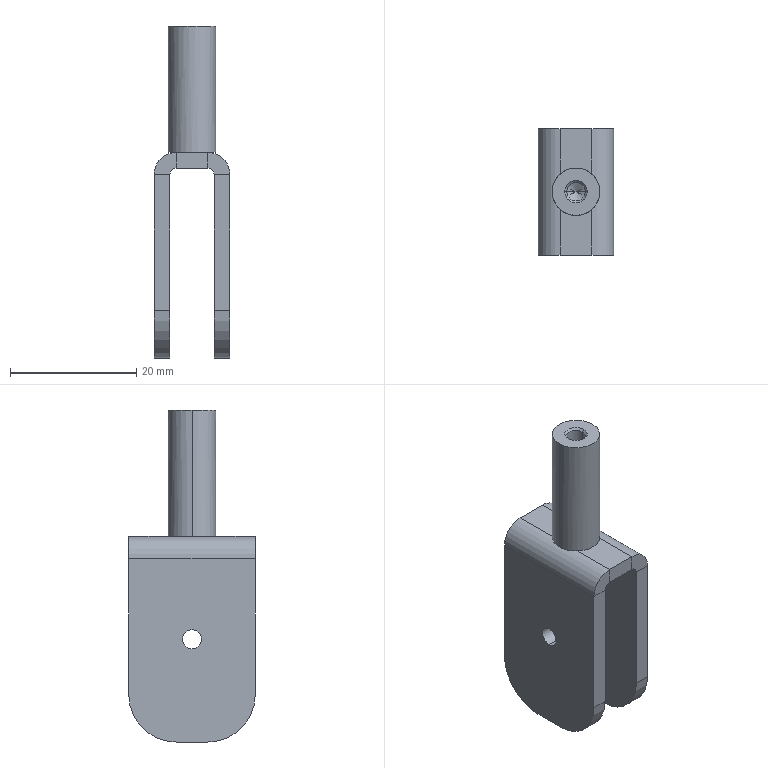Part | SolidWorks | features Cut 1, Fillet 1, FlatPattern 1, HoleWzd 1, ICE 1, SMBaseFlange 1, SheetMetal 1 | 1 solid | 42 faces | box 12 x 20 x 52.5 mm | volume 4162 mm3 | plane 22 | cylinder 16 | cone 4 | commonest cylinder face diameters 3 x4 15 x4 2 x2 2.9 x2 7 x2 7.5 x2
STEP:
#1=CARTESIAN_POINT('',(-1.45,10.,22.175));
#2=VERTEX_POINT('',#1);
#3=CARTESIAN_POINT('',(1.45,10.,22.175));
#4=VERTEX_POINT('',#3);
#5=CARTESIAN_POINT('',(0.,10.,22.175));
#6=DIRECTION('',(0.,0.,1.));
#7=DIRECTION('',(1.,0.,0.));
#8=AXIS2_PLACEMENT_3D('',#5,#6,#7);
#9=CIRCLE('',#8,1.45);
#10=EDGE_CURVE('',#2,#4,#9,.T.);
#11=ORIENTED_EDGE('',*,*,#10,.F.);
#12=CARTESIAN_POINT('',(-1.775,10.,22.5));
#13=VERTEX_POINT('',#12);
#14=CARTESIAN_POINT('',(-1.775,10.,22.5));
#15=DIRECTION('',(-0.7071,0.,0.7071));
#16=VECTOR('',#15,1000.);
#17=LINE('',#14,#16);
#18=EDGE_CURVE('',#2,#13,#17,.T.);
#19=ORIENTED_EDGE('',*,*,#18,.T.);
#20=CARTESIAN_POINT('',(1.775,10.,22.5));
#21=VERTEX_POINT('',#20);
#22=CARTESIAN_POINT('',(0.,10.,22.5));
#23=DIRECTION('',(0.,0.,1.));
#24=DIRECTION('',(1.,0.,0.));
#25=AXIS2_PLACEMENT_3D('',#22,#23,#24);
#26=CIRCLE('',#25,1.775);
#27=EDGE_CURVE('',#13,#21,#26,.T.);
#28=ORIENTED_EDGE('',*,*,#27,.T.);
#29=CARTESIAN_POINT('',(1.775,10.,22.5));
#30=DIRECTION('',(0.7071,0.,0.7071));
#31=VECTOR('',#30,1000.);
#32=LINE('',#29,#31);
#33=EDGE_CURVE('',#4,#21,#32,.T.);
#34=ORIENTED_EDGE('',*,*,#33,.F.);
#35=EDGE_LOOP('',(#11,#19,#28,#34));
#36=FACE_OUTER_BOUND('',#35,.T.);
#37=CARTESIAN_POINT('',(0.,10.,22.5));
#38=DIRECTION('',(0.,0.,1.));
#39=DIRECTION('',(1.,0.,0.));
#40=AXIS2_PLACEMENT_3D('',#37,#38,#39);
#41=CONICAL_SURFACE('',#40,1.775,0.7854);
#42=ADVANCED_FACE('',(#36),#41,.F.);
#43=CARTESIAN_POINT('',(-1.45,10.,12.5));
#44=VERTEX_POINT('',#43);
#45=CARTESIAN_POINT('',(1.45,10.,12.5));
#46=VERTEX_POINT('',#45);
#47=CARTESIAN_POINT('',(0.,10.,12.5));
#48=DIRECTION('',(0.,0.,1.));
#49=DIRECTION('',(1.,0.,0.));
#50=AXIS2_PLACEMENT_3D('',#47,#48,#49);
#51=CIRCLE('',#50,1.45);
#52=EDGE_CURVE('',#44,#46,#51,.T.);
#53=ORIENTED_EDGE('',*,*,#52,.F.);
#54=CARTESIAN_POINT('',(-1.45,10.,22.5));
#55=DIRECTION('',(0.,0.,1.));
#56=VECTOR('',#55,1000.);
#57=LINE('',#54,#56);
#58=EDGE_CURVE('',#44,#2,#57,.T.);
#59=ORIENTED_EDGE('',*,*,#58,.T.);
#60=ORIENTED_EDGE('',*,*,#10,.T.);
#61=CARTESIAN_POINT('',(1.45,10.,22.5));
#62=DIRECTION('',(0.,0.,1.));
#63=VECTOR('',#62,1000.);
#64=LINE('',#61,#63);
#65=EDGE_CURVE('',#46,#4,#64,.T.);
#66=ORIENTED_EDGE('',*,*,#65,.F.);
#67=EDGE_LOOP('',(#53,#59,#60,#66));
#68=FACE_OUTER_BOUND('',#67,.T.);
#69=CARTESIAN_POINT('',(0.,10.,22.5));
#70=DIRECTION('',(0.,0.,1.));
#71=DIRECTION('',(1.,0.,0.));
#72=AXIS2_PLACEMENT_3D('',#69,#70,#71);
#73=CYLINDRICAL_SURFACE('',#72,1.45);
#74=ADVANCED_FACE('',(#68),#73,.F.);
#75=CARTESIAN_POINT('',(0.,10.,11.629));
#76=VERTEX_POINT('',#75);
#77=CARTESIAN_POINT('',(1.45,10.,12.5));
#78=DIRECTION('',(0.8572,0.,0.515));
#79=VECTOR('',#78,1000.);
#80=LINE('',#77,#79);
#81=EDGE_CURVE('',#76,#46,#80,.T.);
#82=ORIENTED_EDGE('',*,*,#81,.F.);
#83=CARTESIAN_POINT('',(-1.45,10.,12.5));
#84=DIRECTION('',(-0.8572,0.,0.515));
#85=VECTOR('',#84,1000.);
#86=LINE('',#83,#85);
#87=EDGE_CURVE('',#76,#44,#86,.T.);
#88=ORIENTED_EDGE('',*,*,#87,.T.);
#89=ORIENTED_EDGE('',*,*,#52,.T.);
#90=EDGE_LOOP('',(#82,#88,#89));
#91=FACE_OUTER_BOUND('',#90,.T.);
#92=CARTESIAN_POINT('',(0.,10.,12.5));
#93=DIRECTION('',(0.,0.,1.));
#94=DIRECTION('',(1.,0.,0.));
#95=AXIS2_PLACEMENT_3D('',#92,#93,#94);
#96=CONICAL_SURFACE('',#95,1.45,1.03);
#97=ADVANCED_FACE('',(#91),#96,.F.);
#98=CARTESIAN_POINT('',(-6.,10.,-12.25));
#99=VERTEX_POINT('',#98);
#100=CARTESIAN_POINT('',(-6.,10.,-15.25));
#101=VERTEX_POINT('',#100);
#102=CARTESIAN_POINT('',(-6.,10.,-13.75));
#103=DIRECTION('',(1.,0.,0.));
#104=DIRECTION('',(0.,0.,1.));
#105=AXIS2_PLACEMENT_3D('',#102,#103,#104);
#106=CIRCLE('',#105,1.5);
#107=EDGE_CURVE('',#99,#101,#106,.T.);
#108=ORIENTED_EDGE('',*,*,#107,.F.);
#109=CARTESIAN_POINT('',(-3.5,10.,-12.25));
#110=VERTEX_POINT('',#109);
#111=CARTESIAN_POINT('',(-10.243,10.,-12.25));
#112=DIRECTION('',(1.,0.,0.));
#113=VECTOR('',#112,1000.);
#114=LINE('',#111,#113);
#115=EDGE_CURVE('',#99,#110,#114,.T.);
#116=ORIENTED_EDGE('',*,*,#115,.T.);
#117=CARTESIAN_POINT('',(-3.5,10.,-15.25));
#118=VERTEX_POINT('',#117);
#119=CARTESIAN_POINT('',(-3.5,10.,-13.75));
#120=DIRECTION('',(-1.,0.,0.));
#121=DIRECTION('',(0.,0.,1.));
#122=AXIS2_PLACEMENT_3D('',#119,#120,#121);
#123=CIRCLE('',#122,1.5);
#124=EDGE_CURVE('',#118,#110,#123,.T.);
#125=ORIENTED_EDGE('',*,*,#124,.F.);
#126=CARTESIAN_POINT('',(-10.243,10.,-15.25));
#127=DIRECTION('',(1.,0.,0.));
#128=VECTOR('',#127,1000.);
#129=LINE('',#126,#128);
#130=EDGE_CURVE('',#101,#118,#129,.T.);
#131=ORIENTED_EDGE('',*,*,#130,.F.);
#132=EDGE_LOOP('',(#108,#116,#125,#131));
#133=FACE_OUTER_BOUND('',#132,.T.);
#134=CARTESIAN_POINT('',(-10.243,10.,-13.75));
#135=DIRECTION('',(1.,0.,0.));
#136=DIRECTION('',(0.,0.,-1.));
#137=AXIS2_PLACEMENT_3D('',#134,#135,#136);
#138=CYLINDRICAL_SURFACE('',#137,1.5);
#139=ADVANCED_FACE('',(#133),#138,.F.);
#140=CARTESIAN_POINT('',(3.5,10.,-12.25));
#141=VERTEX_POINT('',#140);
#142=CARTESIAN_POINT('',(3.5,10.,-15.25));
#143=VERTEX_POINT('',#142);
#144=CARTESIAN_POINT('',(3.5,10.,-13.75));
#145=DIRECTION('',(1.,0.,0.));
#146=DIRECTION('',(0.,0.,-1.));
#147=AXIS2_PLACEMENT_3D('',#144,#145,#146);
#148=CIRCLE('',#147,1.5);
#149=EDGE_CURVE('',#141,#143,#148,.T.);
#150=ORIENTED_EDGE('',*,*,#149,.F.);
#151=CARTESIAN_POINT('',(6.,10.,-12.25));
#152=VERTEX_POINT('',#151);
#153=CARTESIAN_POINT('',(-10.243,10.,-12.25));
#154=DIRECTION('',(1.,0.,0.));
#155=VECTOR('',#154,1000.);
#156=LINE('',#153,#155);
#157=EDGE_CURVE('',#141,#152,#156,.T.);
#158=ORIENTED_EDGE('',*,*,#157,.T.);
#159=CARTESIAN_POINT('',(6.,10.,-15.25));
#160=VERTEX_POINT('',#159);
#161=CARTESIAN_POINT('',(6.,10.,-13.75));
#162=DIRECTION('',(1.,0.,0.));
#163=DIRECTION('',(0.,0.,-1.));
#164=AXIS2_PLACEMENT_3D('',#161,#162,#163);
#165=CIRCLE('',#164,1.5);
#166=EDGE_CURVE('',#152,#160,#165,.T.);
#167=ORIENTED_EDGE('',*,*,#166,.T.);
#168=CARTESIAN_POINT('',(-10.243,10.,-15.25));
#169=DIRECTION('',(1.,0.,0.));
#170=VECTOR('',#169,1000.);
#171=LINE('',#168,#170);
#172=EDGE_CURVE('',#143,#160,#171,.T.);
#173=ORIENTED_EDGE('',*,*,#172,.F.);
#174=EDGE_LOOP('',(#150,#158,#167,#173));
#175=FACE_OUTER_BOUND('',#174,.T.);
#176=CARTESIAN_POINT('',(-10.243,10.,-13.75));
#177=DIRECTION('',(1.,0.,0.));
#178=DIRECTION('',(0.,0.,-1.));
#179=AXIS2_PLACEMENT_3D('',#176,#177,#178);
#180=CYLINDRICAL_SURFACE('',#179,1.5);
#181=ADVANCED_FACE('',(#175),#180,.F.);
#182=CARTESIAN_POINT('',(3.75,10.,22.5));
#183=VERTEX_POINT('',#182);
#184=CARTESIAN_POINT('',(-3.75,10.,22.5));
#185=VERTEX_POINT('',#184);
#186=CARTESIAN_POINT('',(0.,10.,22.5));
#187=DIRECTION('',(0.,0.,1.));
#188=DIRECTION('',(1.,0.,0.));
#189=AXIS2_PLACEMENT_3D('',#186,#187,#188);
#190=CIRCLE('',#189,3.75);
#191=EDGE_CURVE('',#183,#185,#190,.T.);
#192=ORIENTED_EDGE('',*,*,#191,.F.);
#193=CARTESIAN_POINT('',(3.75,10.,2.5));
#194=VERTEX_POINT('',#193);
#195=CARTESIAN_POINT('',(3.75,10.,22.5));
#196=DIRECTION('',(0.,0.,-1.));
#197=VECTOR('',#196,1000.);
#198=LINE('',#195,#197);
#199=EDGE_CURVE('',#183,#194,#198,.T.);
#200=ORIENTED_EDGE('',*,*,#199,.T.);
#201=CARTESIAN_POINT('',(2.5,12.795,2.5));
#202=VERTEX_POINT('',#201);
#203=CARTESIAN_POINT('',(0.,10.,2.5));
#204=DIRECTION('',(0.,0.,1.));
#205=DIRECTION('',(1.,0.,0.));
#206=AXIS2_PLACEMENT_3D('',#203,#204,#205);
#207=CIRCLE('',#206,3.75);
#208=EDGE_CURVE('',#194,#202,#207,.T.);
#209=ORIENTED_EDGE('',*,*,#208,.T.);
#210=CARTESIAN_POINT('',(-2.5,12.795,2.5));
#211=VERTEX_POINT('',#210);
#212=CARTESIAN_POINT('',(0.,10.,2.5));
#213=DIRECTION('',(0.,0.,1.));
#214=DIRECTION('',(1.,0.,0.));
#215=AXIS2_PLACEMENT_3D('',#212,#213,#214);
#216=CIRCLE('',#215,3.75);
#217=EDGE_CURVE('',#202,#211,#216,.T.);
#218=ORIENTED_EDGE('',*,*,#217,.T.);
#219=CARTESIAN_POINT('',(-3.75,10.,2.5));
#220=VERTEX_POINT('',#219);
#221=CARTESIAN_POINT('',(0.,10.,2.5));
#222=DIRECTION('',(0.,0.,1.));
#223=DIRECTION('',(1.,0.,0.));
#224=AXIS2_PLACEMENT_3D('',#221,#222,#223);
#225=CIRCLE('',#224,3.75);
#226=EDGE_CURVE('',#211,#220,#225,.T.);
#227=ORIENTED_EDGE('',*,*,#226,.T.);
#228=CARTESIAN_POINT('',(-3.75,10.,22.5));
#229=DIRECTION('',(0.,0.,-1.));
#230=VECTOR('',#229,1000.);
#231=LINE('',#228,#230);
#232=EDGE_CURVE('',#185,#220,#231,.T.);
#233=ORIENTED_EDGE('',*,*,#232,.F.);
#234=EDGE_LOOP('',(#192,#200,#209,#218,#227,#233));
#235=FACE_OUTER_BOUND('',#234,.T.);
#236=CARTESIAN_POINT('',(0.,10.,22.5));
#237=DIRECTION('',(0.,0.,-1.));
#238=DIRECTION('',(-1.,0.,0.));
#239=AXIS2_PLACEMENT_3D('',#236,#237,#238);
#240=CYLINDRICAL_SURFACE('',#239,3.75);
#241=ADVANCED_FACE('',(#235),#240,.T.);
#242=CARTESIAN_POINT('',(2.5,7.205,2.5));
#243=VERTEX_POINT('',#242);
#244=CARTESIAN_POINT('',(2.5,0.,2.5));
#245=VERTEX_POINT('',#244);
#246=CARTESIAN_POINT('',(2.5,20.,2.5));
#247=DIRECTION('',(0.,-1.,0.));
#248=VECTOR('',#247,1000.);
#249=LINE('',#246,#248);
#250=EDGE_CURVE('',#243,#245,#249,.T.);
#251=ORIENTED_EDGE('',*,*,#250,.F.);
#252=CARTESIAN_POINT('',(-2.5,7.205,2.5));
#253=VERTEX_POINT('',#252);
#254=CARTESIAN_POINT('',(0.,10.,2.5));
#255=DIRECTION('',(0.,0.,1.));
#256=DIRECTION('',(1.,0.,0.));
#257=AXIS2_PLACEMENT_3D('',#254,#255,#256);
#258=CIRCLE('',#257,3.75);
#259=EDGE_CURVE('',#253,#243,#258,.T.);
#260=ORIENTED_EDGE('',*,*,#259,.F.);
#261=CARTESIAN_POINT('',(-2.5,0.,2.5));
#262=VERTEX_POINT('',#261);
#263=CARTESIAN_POINT('',(-2.5,20.,2.5));
#264=DIRECTION('',(0.,-1.,0.));
#265=VECTOR('',#264,1000.);
#266=LINE('',#263,#265);
#267=EDGE_CURVE('',#253,#262,#266,.T.);
#268=ORIENTED_EDGE('',*,*,#267,.T.);
#269=CARTESIAN_POINT('',(-3.5,0.,2.5));
#270=DIRECTION('',(-1.,0.,0.));
#271=VECTOR('',#270,1000.);
#272=LINE('',#269,#271);
#273=EDGE_CURVE('',#245,#262,#272,.T.);
#274=ORIENTED_EDGE('',*,*,#273,.F.);
#275=EDGE_LOOP('',(#251,#260,#268,#274));
#276=FACE_OUTER_BOUND('',#275,.T.);
#277=CARTESIAN_POINT('',(-3.5,20.,2.5));
#278=DIRECTION('',(0.,0.,1.));
#279=DIRECTION('',(1.,0.,0.));
#280=AXIS2_PLACEMENT_3D('',#277,#278,#279);
#281=PLANE('',#280);
#282=ADVANCED_FACE('',(#276),#281,.T.);
#283=CARTESIAN_POINT('',(3.5,20.,-1.));
#284=VERTEX_POINT('',#283);
#285=CARTESIAN_POINT('',(6.,20.,-1.));
#286=VERTEX_POINT('',#285);
#287=CARTESIAN_POINT('',(3.5,20.,-1.));
#288=DIRECTION('',(1.,0.,0.));
#289=VECTOR('',#288,1000.);
#290=LINE('',#287,#289);
#291=EDGE_CURVE('',#284,#286,#290,.T.);
#292=ORIENTED_EDGE('',*,*,#291,.F.);
#293=CARTESIAN_POINT('',(2.5,20.,0.));
#294=VERTEX_POINT('',#293);
#295=CARTESIAN_POINT('',(2.5,20.,-1.));
#296=DIRECTION('',(0.,-1.,0.));
#297=DIRECTION('',(0.,0.,1.));
#298=AXIS2_PLACEMENT_3D('',#295,#296,#297);
#299=CIRCLE('',#298,1.);
#300=EDGE_CURVE('',#284,#294,#299,.T.);
#301=ORIENTED_EDGE('',*,*,#300,.T.);
#302=CARTESIAN_POINT('',(2.5,20.,2.5));
#303=VERTEX_POINT('',#302);
#304=CARTESIAN_POINT('',(2.5,20.,2.5));
#305=DIRECTION('',(0.,0.,-1.));
#306=VECTOR('',#305,1000.);
#307=LINE('',#304,#306);
#308=EDGE_CURVE('',#303,#294,#307,.T.);
#309=ORIENTED_EDGE('',*,*,#308,.F.);
#310=CARTESIAN_POINT('',(2.5,20.,-1.));
#311=DIRECTION('',(0.,-1.,0.));
#312=DIRECTION('',(1.,0.,0.));
#313=AXIS2_PLACEMENT_3D('',#310,#311,#312);
#314=CIRCLE('',#313,3.5);
#315=EDGE_CURVE('',#286,#303,#314,.T.);
#316=ORIENTED_EDGE('',*,*,#315,.F.);
#317=EDGE_LOOP('',(#292,#301,#309,#316));
#318=FACE_OUTER_BOUND('',#317,.T.);
#319=CARTESIAN_POINT('',(3.5,20.,-1.));
#320=DIRECTION('',(0.,1.,0.));
#321=DIRECTION('',(0.,0.,1.));
#322=AXIS2_PLACEMENT_3D('',#319,#320,#321);
#323=PLANE('',#322);
#324=ADVANCED_FACE('',(#318),#323,.T.);
#325=CARTESIAN_POINT('',(6.,20.,-22.5));
#326=VERTEX_POINT('',#325);
#327=CARTESIAN_POINT('',(6.,20.,0.));
#328=DIRECTION('',(0.,0.,1.));
#329=VECTOR('',#328,1000.);
#330=LINE('',#327,#329);
#331=EDGE_CURVE('',#326,#286,#330,.T.);
#332=ORIENTED_EDGE('',*,*,#331,.F.);
#333=CARTESIAN_POINT('',(3.5,20.,-22.5));
#334=VERTEX_POINT('',#333);
#335=CARTESIAN_POINT('',(2.5,20.,-22.5));
#336=DIRECTION('',(-1.,0.,0.));
#337=VECTOR('',#336,1000.);
#338=LINE('',#335,#337);
#339=EDGE_CURVE('',#326,#334,#338,.T.);
#340=ORIENTED_EDGE('',*,*,#339,.T.);
#341=CARTESIAN_POINT('',(3.5,20.,0.));
#342=DIRECTION('',(0.,0.,1.));
#343=VECTOR('',#342,1000.);
#344=LINE('',#341,#343);
#345=EDGE_CURVE('',#334,#284,#344,.T.);
#346=ORIENTED_EDGE('',*,*,#345,.T.);
#347=ORIENTED_EDGE('',*,*,#291,.T.);
#348=EDGE_LOOP('',(#332,#340,#346,#347));
#349=FACE_OUTER_BOUND('',#348,.T.);
#350=CARTESIAN_POINT('',(2.5,20.,2.5));
#351=DIRECTION('',(0.,1.,0.));
#352=DIRECTION('',(0.,0.,1.));
#353=AXIS2_PLACEMENT_3D('',#350,#351,#352);
#354=PLANE('',#353);
#355=ADVANCED_FACE('',(#349),#354,.T.);
#356=CARTESIAN_POINT('',(2.5,0.,0.));
#357=VERTEX_POINT('',#356);
#358=CARTESIAN_POINT('',(2.5,0.,0.));
#359=DIRECTION('',(0.,0.,1.));
#360=VECTOR('',#359,1000.);
#361=LINE('',#358,#360);
#362=EDGE_CURVE('',#357,#245,#361,.T.);
#363=ORIENTED_EDGE('',*,*,#362,.F.);
#364=CARTESIAN_POINT('',(3.5,0.,-1.));
#365=VERTEX_POINT('',#364);
#366=CARTESIAN_POINT('',(2.5,0.,-1.));
#367=DIRECTION('',(0.,-1.,0.));
#368=DIRECTION('',(0.,0.,1.));
#369=AXIS2_PLACEMENT_3D('',#366,#367,#368);
#370=CIRCLE('',#369,1.);
#371=EDGE_CURVE('',#365,#357,#370,.T.);
#372=ORIENTED_EDGE('',*,*,#371,.F.);
#373=CARTESIAN_POINT('',(6.,0.,-1.));
#374=VERTEX_POINT('',#373);
#375=CARTESIAN_POINT('',(6.,0.,-1.));
#376=DIRECTION('',(-1.,0.,0.));
#377=VECTOR('',#376,1000.);
#378=LINE('',#375,#377);
#379=EDGE_CURVE('',#374,#365,#378,.T.);
#380=ORIENTED_EDGE('',*,*,#379,.F.);
#381=CARTESIAN_POINT('',(2.5,0.,-1.));
#382=DIRECTION('',(0.,-1.,0.));
#383=DIRECTION('',(1.,0.,0.));
#384=AXIS2_PLACEMENT_3D('',#381,#382,#383);
#385=CIRCLE('',#384,3.5);
#386=EDGE_CURVE('',#374,#245,#385,.T.);
#387=ORIENTED_EDGE('',*,*,#386,.T.);
#388=EDGE_LOOP('',(#363,#372,#380,#387));
#389=FACE_OUTER_BOUND('',#388,.T.);
#390=CARTESIAN_POINT('',(2.5,0.,0.));
#391=DIRECTION('',(0.,-1.,0.));
#392=DIRECTION('',(0.,0.,-1.));
#393=AXIS2_PLACEMENT_3D('',#390,#391,#392);
#394=PLANE('',#393);
#395=ADVANCED_FACE('',(#389),#394,.T.);
#396=CARTESIAN_POINT('',(-2.5,0.,0.));
#397=VERTEX_POINT('',#396);
#398=CARTESIAN_POINT('',(-3.5,0.,0.));
#399=DIRECTION('',(-1.,0.,0.));
#400=VECTOR('',#399,1000.);
#401=LINE('',#398,#400);
#402=EDGE_CURVE('',#357,#397,#401,.T.);
#403=ORIENTED_EDGE('',*,*,#402,.F.);
#404=ORIENTED_EDGE('',*,*,#362,.T.);
#405=ORIENTED_EDGE('',*,*,#273,.T.);
#406=CARTESIAN_POINT('',(-2.5,0.,2.5));
#407=DIRECTION('',(0.,0.,-1.));
#408=VECTOR('',#407,1000.);
#409=LINE('',#406,#408);
#410=EDGE_CURVE('',#262,#397,#409,.T.);
#411=ORIENTED_EDGE('',*,*,#410,.T.);
#412=EDGE_LOOP('',(#403,#404,#405,#411));
#413=FACE_OUTER_BOUND('',#412,.T.);
#414=CARTESIAN_POINT('',(6.,0.,-1.));
#415=DIRECTION('',(0.,-1.,0.));
#416=DIRECTION('',(0.,0.,-1.));
#417=AXIS2_PLACEMENT_3D('',#414,#415,#416);
#418=PLANE('',#417);
#419=ADVANCED_FACE('',(#413),#418,.T.);
#420=CARTESIAN_POINT('',(-2.5,20.,0.));
#421=VERTEX_POINT('',#420);
#422=CARTESIAN_POINT('',(-2.5,20.,2.5));
#423=VERTEX_POINT('',#422);
#424=CARTESIAN_POINT('',(-2.5,20.,0.));
#425=DIRECTION('',(0.,0.,1.));
#426=VECTOR('',#425,1000.);
#427=LINE('',#424,#426);
#428=EDGE_CURVE('',#421,#423,#427,.T.);
#429=ORIENTED_EDGE('',*,*,#428,.F.);
#430=CARTESIAN_POINT('',(-3.5,20.,-1.));
#431=VERTEX_POINT('',#430);
#432=CARTESIAN_POINT('',(-2.5,20.,-1.));
#433=DIRECTION('',(0.,-1.,0.));
#434=DIRECTION('',(0.,0.,1.));
#435=AXIS2_PLACEMENT_3D('',#432,#433,#434);
#436=CIRCLE('',#435,1.);
#437=EDGE_CURVE('',#421,#431,#436,.T.);
#438=ORIENTED_EDGE('',*,*,#437,.T.);
#439=CARTESIAN_POINT('',(-6.,20.,-1.));
#440=VERTEX_POINT('',#439);
#441=CARTESIAN_POINT('',(-6.,20.,-1.));
#442=DIRECTION('',(1.,0.,0.));
#443=VECTOR('',#442,1000.);
#444=LINE('',#441,#443);
#445=EDGE_CURVE('',#440,#431,#444,.T.);
#446=ORIENTED_EDGE('',*,*,#445,.F.);
#447=CARTESIAN_POINT('',(-2.5,20.,-1.));
#448=DIRECTION('',(0.,-1.,0.));
#449=DIRECTION('',(1.,0.,0.));
#450=AXIS2_PLACEMENT_3D('',#447,#448,#449);
#451=CIRCLE('',#450,3.5);
#452=EDGE_CURVE('',#423,#440,#451,.T.);
#453=ORIENTED_EDGE('',*,*,#452,.F.);
#454=EDGE_LOOP('',(#429,#438,#446,#453));
#455=FACE_OUTER_BOUND('',#454,.T.);
#456=CARTESIAN_POINT('',(-2.5,20.,0.));
#457=DIRECTION('',(0.,1.,0.));
#458=DIRECTION('',(0.,0.,1.));
#459=AXIS2_PLACEMENT_3D('',#456,#457,#458);
#460=PLANE('',#459);
#461=ADVANCED_FACE('',(#455),#460,.T.);
#462=CARTESIAN_POINT('',(-3.5,20.,0.));
#463=DIRECTION('',(-1.,0.,0.));
#464=VECTOR('',#463,1000.);
#465=LINE('',#462,#464);
#466=EDGE_CURVE('',#294,#421,#465,.T.);
#467=ORIENTED_EDGE('',*,*,#466,.T.);
#468=ORIENTED_EDGE('',*,*,#428,.T.);
#469=CARTESIAN_POINT('',(-3.5,20.,2.5));
#470=DIRECTION('',(-1.,0.,0.));
#471=VECTOR('',#470,1000.);
#472=LINE('',#469,#471);
#473=EDGE_CURVE('',#303,#423,#472,.T.);
#474=ORIENTED_EDGE('',*,*,#473,.F.);
#475=ORIENTED_EDGE('',*,*,#308,.T.);
#476=EDGE_LOOP('',(#467,#468,#474,#475));
#477=FACE_OUTER_BOUND('',#476,.T.);
#478=CARTESIAN_POINT('',(-6.,20.,-1.));
#479=DIRECTION('',(0.,1.,0.));
#480=DIRECTION('',(0.,0.,1.));
#481=AXIS2_PLACEMENT_3D('',#478,#479,#480);
#482=PLANE('',#481);
#483=ADVANCED_FACE('',(#477),#482,.T.);
#484=CARTESIAN_POINT('',(-3.5,0.,-1.));
#485=VERTEX_POINT('',#484);
#486=CARTESIAN_POINT('',(-6.,0.,-1.));
#487=VERTEX_POINT('',#486);
#488=CARTESIAN_POINT('',(-3.5,0.,-1.));
#489=DIRECTION('',(-1.,0.,0.));
#490=VECTOR('',#489,1000.);
#491=LINE('',#488,#490);
#492=EDGE_CURVE('',#485,#487,#491,.T.);
#493=ORIENTED_EDGE('',*,*,#492,.F.);
#494=CARTESIAN_POINT('',(-2.5,0.,-1.));
#495=DIRECTION('',(0.,-1.,0.));
#496=DIRECTION('',(0.,0.,1.));
#497=AXIS2_PLACEMENT_3D('',#494,#495,#496);
#498=CIRCLE('',#497,1.);
#499=EDGE_CURVE('',#397,#485,#498,.T.);
#500=ORIENTED_EDGE('',*,*,#499,.F.);
#501=ORIENTED_EDGE('',*,*,#410,.F.);
#502=CARTESIAN_POINT('',(-2.5,0.,-1.));
#503=DIRECTION('',(0.,-1.,0.));
#504=DIRECTION('',(1.,0.,0.));
#505=AXIS2_PLACEMENT_3D('',#502,#503,#504);
#506=CIRCLE('',#505,3.5);
#507=EDGE_CURVE('',#262,#487,#506,.T.);
#508=ORIENTED_EDGE('',*,*,#507,.T.);
#509=EDGE_LOOP('',(#493,#500,#501,#508));
#510=FACE_OUTER_BOUND('',#509,.T.);
#511=CARTESIAN_POINT('',(-3.5,0.,-1.));
#512=DIRECTION('',(0.,-1.,0.));
#513=DIRECTION('',(0.,0.,-1.));
#514=AXIS2_PLACEMENT_3D('',#511,#512,#513);
#515=PLANE('',#514);
#516=ADVANCED_FACE('',(#510),#515,.T.);
#517=CARTESIAN_POINT('',(-6.,0.,-22.5));
#518=VERTEX_POINT('',#517);
#519=CARTESIAN_POINT('',(-6.,0.,0.));
#520=DIRECTION('',(0.,0.,-1.));
#521=VECTOR('',#520,1000.);
#522=LINE('',#519,#521);
#523=EDGE_CURVE('',#487,#518,#522,.T.);
#524=ORIENTED_EDGE('',*,*,#523,.T.);
#525=CARTESIAN_POINT('',(-3.5,0.,-22.5));
#526=VERTEX_POINT('',#525);
#527=CARTESIAN_POINT('',(-2.5,0.,-22.5));
#528=DIRECTION('',(1.,0.,0.));
#529=VECTOR('',#528,1000.);
#530=LINE('',#527,#529);
#531=EDGE_CURVE('',#518,#526,#530,.T.);
#532=ORIENTED_EDGE('',*,*,#531,.T.);
#533=CARTESIAN_POINT('',(-3.5,0.,0.));
#534=DIRECTION('',(0.,0.,-1.));
#535=VECTOR('',#534,1000.);
#536=LINE('',#533,#535);
#537=EDGE_CURVE('',#485,#526,#536,.T.);
#538=ORIENTED_EDGE('',*,*,#537,.F.);
#539=ORIENTED_EDGE('',*,*,#492,.T.);
#540=EDGE_LOOP('',(#524,#532,#538,#539));
#541=FACE_OUTER_BOUND('',#540,.T.);
#542=CARTESIAN_POINT('',(-2.5,0.,2.5));
#543=DIRECTION('',(0.,-1.,0.));
#544=DIRECTION('',(0.,0.,-1.));
#545=AXIS2_PLACEMENT_3D('',#542,#543,#544);
#546=PLANE('',#545);
#547=ADVANCED_FACE('',(#541),#546,.T.);
#548=ORIENTED_EDGE('',*,*,#124,.T.);
#549=CARTESIAN_POINT('',(-3.5,10.,-13.75));
#550=DIRECTION('',(-1.,0.,0.));
#551=DIRECTION('',(0.,0.,1.));
#552=AXIS2_PLACEMENT_3D('',#549,#550,#551);
#553=CIRCLE('',#552,1.5);
#554=EDGE_CURVE('',#110,#118,#553,.T.);
#555=ORIENTED_EDGE('',*,*,#554,.T.);
#556=EDGE_LOOP('',(#548,#555));
#557=FACE_BOUND('',#556,.T.);
#558=ORIENTED_EDGE('',*,*,#537,.T.);
#559=CARTESIAN_POINT('',(-3.5,7.5,-30.));
#560=VERTEX_POINT('',#559);
#561=CARTESIAN_POINT('',(-3.5,7.5,-22.5));
#562=DIRECTION('',(1.,0.,0.));
#563=DIRECTION('',(0.,0.,1.));
#564=AXIS2_PLACEMENT_3D('',#561,#562,#563);
#565=CIRCLE('',#564,7.5);
#566=EDGE_CURVE('',#526,#560,#565,.T.);
#567=ORIENTED_EDGE('',*,*,#566,.T.);
#568=CARTESIAN_POINT('',(-3.5,12.5,-30.));
#569=VERTEX_POINT('',#568);
#570=CARTESIAN_POINT('',(-3.5,20.,-30.));
#571=DIRECTION('',(0.,-1.,0.));
#572=VECTOR('',#571,1000.);
#573=LINE('',#570,#572);
#574=EDGE_CURVE('',#569,#560,#573,.T.);
#575=ORIENTED_EDGE('',*,*,#574,.F.);
#576=CARTESIAN_POINT('',(-3.5,20.,-22.5));
#577=VERTEX_POINT('',#576);
#578=CARTESIAN_POINT('',(-3.5,12.5,-22.5));
#579=DIRECTION('',(1.,0.,0.));
#580=DIRECTION('',(0.,0.,1.));
#581=AXIS2_PLACEMENT_3D('',#578,#579,#580);
#582=CIRCLE('',#581,7.5);
#583=EDGE_CURVE('',#569,#577,#582,.T.);
#584=ORIENTED_EDGE('',*,*,#583,.T.);
#585=CARTESIAN_POINT('',(-3.5,20.,0.));
#586=DIRECTION('',(0.,0.,-1.));
#587=VECTOR('',#586,1000.);
#588=LINE('',#585,#587);
#589=EDGE_CURVE('',#431,#577,#588,.T.);
#590=ORIENTED_EDGE('',*,*,#589,.F.);
#591=CARTESIAN_POINT('',(-3.5,20.,-1.));
#592=DIRECTION('',(0.,-1.,0.));
#593=VECTOR('',#592,1000.);
#594=LINE('',#591,#593);
#595=EDGE_CURVE('',#431,#485,#594,.T.);
#596=ORIENTED_EDGE('',*,*,#595,.T.);
#597=EDGE_LOOP('',(#558,#567,#575,#584,#590,#596));
#598=FACE_OUTER_BOUND('',#597,.T.);
#599=CARTESIAN_POINT('',(-3.5,20.,0.));
#600=DIRECTION('',(-1.,0.,0.));
#601=DIRECTION('',(0.,0.,1.));
#602=AXIS2_PLACEMENT_3D('',#599,#600,#601);
#603=PLANE('',#602);
#604=ADVANCED_FACE('',(#557,#598),#603,.F.);
#605=ORIENTED_EDGE('',*,*,#574,.T.);
#606=CARTESIAN_POINT('',(-6.,7.5,-30.));
#607=VERTEX_POINT('',#606);
#608=CARTESIAN_POINT('',(-6.,7.5,-30.));
#609=DIRECTION('',(-1.,0.,0.));
#610=VECTOR('',#609,1000.);
#611=LINE('',#608,#610);
#612=EDGE_CURVE('',#560,#607,#611,.T.);
#613=ORIENTED_EDGE('',*,*,#612,.T.);
#614=CARTESIAN_POINT('',(-6.,12.5,-30.));
#615=VERTEX_POINT('',#614);
#616=CARTESIAN_POINT('',(-6.,20.,-30.));
#617=DIRECTION('',(0.,-1.,0.));
#618=VECTOR('',#617,1000.);
#619=LINE('',#616,#618);
#620=EDGE_CURVE('',#615,#607,#619,.T.);
#621=ORIENTED_EDGE('',*,*,#620,.F.);
#622=CARTESIAN_POINT('',(-6.,12.5,-30.));
#623=DIRECTION('',(1.,0.,0.));
#624=VECTOR('',#623,1000.);
#625=LINE('',#622,#624);
#626=EDGE_CURVE('',#615,#569,#625,.T.);
#627=ORIENTED_EDGE('',*,*,#626,.T.);
#628=EDGE_LOOP('',(#605,#613,#621,#627));
#629=FACE_OUTER_BOUND('',#628,.T.);
#630=CARTESIAN_POINT('',(-6.,20.,-30.));
#631=DIRECTION('',(0.,0.,-1.));
#632=DIRECTION('',(-1.,0.,0.));
#633=AXIS2_PLACEMENT_3D('',#630,#631,#632);
#634=PLANE('',#633);
#635=ADVANCED_FACE('',(#629),#634,.T.);
#636=CARTESIAN_POINT('',(-6.,10.,-13.75));
#637=DIRECTION('',(1.,0.,0.));
#638=DIRECTION('',(0.,0.,1.));
#639=AXIS2_PLACEMENT_3D('',#636,#637,#638);
#640=CIRCLE('',#639,1.5);
#641=EDGE_CURVE('',#101,#99,#640,.T.);
#642=ORIENTED_EDGE('',*,*,#641,.T.);
#643=ORIENTED_EDGE('',*,*,#107,.T.);
#644=EDGE_LOOP('',(#642,#643));
#645=FACE_BOUND('',#644,.T.);
#646=ORIENTED_EDGE('',*,*,#620,.T.);
#647=CARTESIAN_POINT('',(-6.,7.5,-22.5));
#648=DIRECTION('',(-1.,0.,0.));
#649=DIRECTION('',(0.,0.,1.));
#650=AXIS2_PLACEMENT_3D('',#647,#648,#649);
#651=CIRCLE('',#650,7.5);
#652=EDGE_CURVE('',#607,#518,#651,.T.);
#653=ORIENTED_EDGE('',*,*,#652,.T.);
#654=ORIENTED_EDGE('',*,*,#523,.F.);
#655=CARTESIAN_POINT('',(-6.,20.,-1.));
#656=DIRECTION('',(0.,-1.,0.));
#657=VECTOR('',#656,1000.);
#658=LINE('',#655,#657);
#659=EDGE_CURVE('',#440,#487,#658,.T.);
#660=ORIENTED_EDGE('',*,*,#659,.F.);
#661=CARTESIAN_POINT('',(-6.,20.,-22.5));
#662=VERTEX_POINT('',#661);
#663=CARTESIAN_POINT('',(-6.,20.,0.));
#664=DIRECTION('',(0.,0.,-1.));
#665=VECTOR('',#664,1000.);
#666=LINE('',#663,#665);
#667=EDGE_CURVE('',#440,#662,#666,.T.);
#668=ORIENTED_EDGE('',*,*,#667,.T.);
#669=CARTESIAN_POINT('',(-6.,12.5,-22.5));
#670=DIRECTION('',(-1.,0.,0.));
#671=DIRECTION('',(0.,0.,1.));
#672=AXIS2_PLACEMENT_3D('',#669,#670,#671);
#673=CIRCLE('',#672,7.5);
#674=EDGE_CURVE('',#662,#615,#673,.T.);
#675=ORIENTED_EDGE('',*,*,#674,.T.);
#676=EDGE_LOOP('',(#646,#653,#654,#660,#668,#675));
#677=FACE_OUTER_BOUND('',#676,.T.);
#678=CARTESIAN_POINT('',(-6.,20.,0.));
#679=DIRECTION('',(-1.,0.,0.));
#680=DIRECTION('',(0.,0.,1.));
#681=AXIS2_PLACEMENT_3D('',#678,#679,#680);
#682=PLANE('',#681);
#683=ADVANCED_FACE('',(#645,#677),#682,.T.);
#684=ORIENTED_EDGE('',*,*,#507,.F.);
#685=ORIENTED_EDGE('',*,*,#267,.F.);
#686=CARTESIAN_POINT('',(-2.5,20.,2.5));
#687=DIRECTION('',(0.,1.,0.));
#688=VECTOR('',#687,1000.);
#689=LINE('',#686,#688);
#690=EDGE_CURVE('',#253,#211,#689,.T.);
#691=ORIENTED_EDGE('',*,*,#690,.T.);
#692=CARTESIAN_POINT('',(-2.5,20.,2.5));
#693=DIRECTION('',(0.,-1.,0.));
#694=VECTOR('',#693,1000.);
#695=LINE('',#692,#694);
#696=EDGE_CURVE('',#423,#211,#695,.T.);
#697=ORIENTED_EDGE('',*,*,#696,.F.);
#698=ORIENTED_EDGE('',*,*,#452,.T.);
#699=ORIENTED_EDGE('',*,*,#659,.T.);
#700=EDGE_LOOP('',(#684,#685,#691,#697,#698,#699));
#701=FACE_OUTER_BOUND('',#700,.T.);
#702=CARTESIAN_POINT('',(-2.5,20.,-1.));
#703=DIRECTION('',(0.,-1.,0.));
#704=DIRECTION('',(0.,0.,-1.));
#705=AXIS2_PLACEMENT_3D('',#702,#703,#704);
#706=CYLINDRICAL_SURFACE('',#705,3.5);
#707=ADVANCED_FACE('',(#701),#706,.T.);
#708=ORIENTED_EDGE('',*,*,#696,.T.);
#709=ORIENTED_EDGE('',*,*,#217,.F.);
#710=CARTESIAN_POINT('',(2.5,20.,2.5));
#711=DIRECTION('',(0.,-1.,0.));
#712=VECTOR('',#711,1000.);
#713=LINE('',#710,#712);
#714=EDGE_CURVE('',#303,#202,#713,.T.);
#715=ORIENTED_EDGE('',*,*,#714,.F.);
#716=ORIENTED_EDGE('',*,*,#473,.T.);
#717=EDGE_LOOP('',(#708,#709,#715,#716));
#718=FACE_OUTER_BOUND('',#717,.T.);
#719=CARTESIAN_POINT('',(-3.5,20.,2.5));
#720=DIRECTION('',(0.,0.,1.));
#721=DIRECTION('',(1.,0.,0.));
#722=AXIS2_PLACEMENT_3D('',#719,#720,#721);
#723=PLANE('',#722);
#724=ADVANCED_FACE('',(#718),#723,.T.);
#725=ORIENTED_EDGE('',*,*,#386,.F.);
#726=CARTESIAN_POINT('',(6.,20.,-1.));
#727=DIRECTION('',(0.,-1.,0.));
#728=VECTOR('',#727,1000.);
#729=LINE('',#726,#728);
#730=EDGE_CURVE('',#286,#374,#729,.T.);
#731=ORIENTED_EDGE('',*,*,#730,.F.);
#732=ORIENTED_EDGE('',*,*,#315,.T.);
#733=ORIENTED_EDGE('',*,*,#714,.T.);
#734=CARTESIAN_POINT('',(2.5,20.,2.5));
#735=DIRECTION('',(0.,-1.,0.));
#736=VECTOR('',#735,1000.);
#737=LINE('',#734,#736);
#738=EDGE_CURVE('',#202,#243,#737,.T.);
#739=ORIENTED_EDGE('',*,*,#738,.T.);
#740=ORIENTED_EDGE('',*,*,#250,.T.);
#741=EDGE_LOOP('',(#725,#731,#732,#733,#739,#740));
#742=FACE_OUTER_BOUND('',#741,.T.);
#743=CARTESIAN_POINT('',(2.5,20.,-1.));
#744=DIRECTION('',(0.,-1.,0.));
#745=DIRECTION('',(0.,0.,-1.));
#746=AXIS2_PLACEMENT_3D('',#743,#744,#745);
#747=CYLINDRICAL_SURFACE('',#746,3.5);
#748=ADVANCED_FACE('',(#742),#747,.T.);
#749=CARTESIAN_POINT('',(6.,10.,-13.75));
#750=DIRECTION('',(1.,0.,0.));
#751=DIRECTION('',(0.,0.,-1.));
#752=AXIS2_PLACEMENT_3D('',#749,#750,#751);
#753=CIRCLE('',#752,1.5);
#754=EDGE_CURVE('',#160,#152,#753,.T.);
#755=ORIENTED_EDGE('',*,*,#754,.F.);
#756=ORIENTED_EDGE('',*,*,#166,.F.);
#757=EDGE_LOOP('',(#755,#756));
#758=FACE_BOUND('',#757,.T.);
#759=CARTESIAN_POINT('',(6.,0.,-22.5));
#760=VERTEX_POINT('',#759);
#761=CARTESIAN_POINT('',(6.,0.,0.));
#762=DIRECTION('',(0.,0.,1.));
#763=VECTOR('',#762,1000.);
#764=LINE('',#761,#763);
#765=EDGE_CURVE('',#760,#374,#764,.T.);
#766=ORIENTED_EDGE('',*,*,#765,.F.);
#767=CARTESIAN_POINT('',(6.,7.5,-30.));
#768=VERTEX_POINT('',#767);
#769=CARTESIAN_POINT('',(6.,7.5,-22.5));
#770=DIRECTION('',(1.,0.,0.));
#771=DIRECTION('',(0.,0.,-1.));
#772=AXIS2_PLACEMENT_3D('',#769,#770,#771);
#773=CIRCLE('',#772,7.5);
#774=EDGE_CURVE('',#760,#768,#773,.T.);
#775=ORIENTED_EDGE('',*,*,#774,.T.);
#776=CARTESIAN_POINT('',(6.,12.5,-30.));
#777=VERTEX_POINT('',#776);
#778=CARTESIAN_POINT('',(6.,20.,-30.));
#779=DIRECTION('',(0.,-1.,0.));
#780=VECTOR('',#779,1000.);
#781=LINE('',#778,#780);
#782=EDGE_CURVE('',#777,#768,#781,.T.);
#783=ORIENTED_EDGE('',*,*,#782,.F.);
#784=CARTESIAN_POINT('',(6.,12.5,-22.5));
#785=DIRECTION('',(1.,0.,0.));
#786=DIRECTION('',(0.,0.,-1.));
#787=AXIS2_PLACEMENT_3D('',#784,#785,#786);
#788=CIRCLE('',#787,7.5);
#789=EDGE_CURVE('',#777,#326,#788,.T.);
#790=ORIENTED_EDGE('',*,*,#789,.T.);
#791=ORIENTED_EDGE('',*,*,#331,.T.);
#792=ORIENTED_EDGE('',*,*,#730,.T.);
#793=EDGE_LOOP('',(#766,#775,#783,#790,#791,#792));
#794=FACE_OUTER_BOUND('',#793,.T.);
#795=CARTESIAN_POINT('',(6.,20.,0.));
#796=DIRECTION('',(1.,0.,0.));
#797=DIRECTION('',(0.,0.,-1.));
#798=AXIS2_PLACEMENT_3D('',#795,#796,#797);
#799=PLANE('',#798);
#800=ADVANCED_FACE('',(#758,#794),#799,.T.);
#801=ORIENTED_EDGE('',*,*,#782,.T.);
#802=CARTESIAN_POINT('',(3.5,7.5,-30.));
#803=VERTEX_POINT('',#802);
#804=CARTESIAN_POINT('',(3.5,7.5,-30.));
#805=DIRECTION('',(-1.,0.,0.));
#806=VECTOR('',#805,1000.);
#807=LINE('',#804,#806);
#808=EDGE_CURVE('',#768,#803,#807,.T.);
#809=ORIENTED_EDGE('',*,*,#808,.T.);
#810=CARTESIAN_POINT('',(3.5,12.5,-30.));
#811=VERTEX_POINT('',#810);
#812=CARTESIAN_POINT('',(3.5,20.,-30.));
#813=DIRECTION('',(0.,-1.,0.));
#814=VECTOR('',#813,1000.);
#815=LINE('',#812,#814);
#816=EDGE_CURVE('',#811,#803,#815,.T.);
#817=ORIENTED_EDGE('',*,*,#816,.F.);
#818=CARTESIAN_POINT('',(3.5,12.5,-30.));
#819=DIRECTION('',(1.,0.,0.));
#820=VECTOR('',#819,1000.);
#821=LINE('',#818,#820);
#822=EDGE_CURVE('',#811,#777,#821,.T.);
#823=ORIENTED_EDGE('',*,*,#822,.T.);
#824=EDGE_LOOP('',(#801,#809,#817,#823));
#825=FACE_OUTER_BOUND('',#824,.T.);
#826=CARTESIAN_POINT('',(3.5,20.,-30.));
#827=DIRECTION('',(0.,0.,-1.));
#828=DIRECTION('',(-1.,0.,0.));
#829=AXIS2_PLACEMENT_3D('',#826,#827,#828);
#830=PLANE('',#829);
#831=ADVANCED_FACE('',(#825),#830,.T.);
#832=CARTESIAN_POINT('',(3.5,10.,-13.75));
#833=DIRECTION('',(1.,0.,0.));
#834=DIRECTION('',(0.,0.,-1.));
#835=AXIS2_PLACEMENT_3D('',#832,#833,#834);
#836=CIRCLE('',#835,1.5);
#837=EDGE_CURVE('',#143,#141,#836,.T.);
#838=ORIENTED_EDGE('',*,*,#837,.T.);
#839=ORIENTED_EDGE('',*,*,#149,.T.);
#840=EDGE_LOOP('',(#838,#839));
#841=FACE_BOUND('',#840,.T.);
#842=ORIENTED_EDGE('',*,*,#816,.T.);
#843=CARTESIAN_POINT('',(3.5,0.,-22.5));
#844=VERTEX_POINT('',#843);
#845=CARTESIAN_POINT('',(3.5,7.5,-22.5));
#846=DIRECTION('',(-1.,0.,0.));
#847=DIRECTION('',(0.,0.,-1.));
#848=AXIS2_PLACEMENT_3D('',#845,#846,#847);
#849=CIRCLE('',#848,7.5);
#850=EDGE_CURVE('',#803,#844,#849,.T.);
#851=ORIENTED_EDGE('',*,*,#850,.T.);
#852=CARTESIAN_POINT('',(3.5,0.,0.));
#853=DIRECTION('',(0.,0.,1.));
#854=VECTOR('',#853,1000.);
#855=LINE('',#852,#854);
#856=EDGE_CURVE('',#844,#365,#855,.T.);
#857=ORIENTED_EDGE('',*,*,#856,.T.);
#858=CARTESIAN_POINT('',(3.5,20.,-1.));
#859=DIRECTION('',(0.,-1.,0.));
#860=VECTOR('',#859,1000.);
#861=LINE('',#858,#860);
#862=EDGE_CURVE('',#284,#365,#861,.T.);
#863=ORIENTED_EDGE('',*,*,#862,.F.);
#864=ORIENTED_EDGE('',*,*,#345,.F.);
#865=CARTESIAN_POINT('',(3.5,12.5,-22.5));
#866=DIRECTION('',(-1.,0.,0.));
#867=DIRECTION('',(0.,0.,-1.));
#868=AXIS2_PLACEMENT_3D('',#865,#866,#867);
#869=CIRCLE('',#868,7.5);
#870=EDGE_CURVE('',#334,#811,#869,.T.);
#871=ORIENTED_EDGE('',*,*,#870,.T.);
#872=EDGE_LOOP('',(#842,#851,#857,#863,#864,#871));
#873=FACE_OUTER_BOUND('',#872,.T.);
#874=CARTESIAN_POINT('',(3.5,20.,0.));
#875=DIRECTION('',(1.,0.,0.));
#876=DIRECTION('',(0.,0.,-1.));
#877=AXIS2_PLACEMENT_3D('',#874,#875,#876);
#878=PLANE('',#877);
#879=ADVANCED_FACE('',(#841,#873),#878,.F.);
#880=ORIENTED_EDGE('',*,*,#371,.T.);
#881=CARTESIAN_POINT('',(2.5,20.,0.));
#882=DIRECTION('',(0.,-1.,0.));
#883=VECTOR('',#882,1000.);
#884=LINE('',#881,#883);
#885=EDGE_CURVE('',#294,#357,#884,.T.);
#886=ORIENTED_EDGE('',*,*,#885,.F.);
#887=ORIENTED_EDGE('',*,*,#300,.F.);
#888=ORIENTED_EDGE('',*,*,#862,.T.);
#889=EDGE_LOOP('',(#880,#886,#887,#888));
#890=FACE_OUTER_BOUND('',#889,.T.);
#891=CARTESIAN_POINT('',(2.5,20.,-1.));
#892=DIRECTION('',(0.,-1.,0.));
#893=DIRECTION('',(0.,0.,-1.));
#894=AXIS2_PLACEMENT_3D('',#891,#892,#893);
#895=CYLINDRICAL_SURFACE('',#894,1.);
#896=ADVANCED_FACE('',(#890),#895,.F.);
#897=ORIENTED_EDGE('',*,*,#402,.T.);
#898=CARTESIAN_POINT('',(-2.5,20.,0.));
#899=DIRECTION('',(0.,-1.,0.));
#900=VECTOR('',#899,1000.);
#901=LINE('',#898,#900);
#902=EDGE_CURVE('',#421,#397,#901,.T.);
#903=ORIENTED_EDGE('',*,*,#902,.F.);
#904=ORIENTED_EDGE('',*,*,#466,.F.);
#905=ORIENTED_EDGE('',*,*,#885,.T.);
#906=EDGE_LOOP('',(#897,#903,#904,#905));
#907=FACE_OUTER_BOUND('',#906,.T.);
#908=CARTESIAN_POINT('',(-3.5,20.,0.));
#909=DIRECTION('',(0.,0.,1.));
#910=DIRECTION('',(1.,0.,0.));
#911=AXIS2_PLACEMENT_3D('',#908,#909,#910);
#912=PLANE('',#911);
#913=ADVANCED_FACE('',(#907),#912,.F.);
#914=ORIENTED_EDGE('',*,*,#499,.T.);
#915=ORIENTED_EDGE('',*,*,#595,.F.);
#916=ORIENTED_EDGE('',*,*,#437,.F.);
#917=ORIENTED_EDGE('',*,*,#902,.T.);
#918=EDGE_LOOP('',(#914,#915,#916,#917));
#919=FACE_OUTER_BOUND('',#918,.T.);
#920=CARTESIAN_POINT('',(-2.5,20.,-1.));
#921=DIRECTION('',(0.,-1.,0.));
#922=DIRECTION('',(0.,0.,-1.));
#923=AXIS2_PLACEMENT_3D('',#920,#921,#922);
#924=CYLINDRICAL_SURFACE('',#923,1.);
#925=ADVANCED_FACE('',(#919),#924,.F.);
#926=ORIENTED_EDGE('',*,*,#589,.T.);
#927=CARTESIAN_POINT('',(-2.5,20.,-22.5));
#928=DIRECTION('',(-1.,0.,0.));
#929=VECTOR('',#928,1000.);
#930=LINE('',#927,#929);
#931=EDGE_CURVE('',#577,#662,#930,.T.);
#932=ORIENTED_EDGE('',*,*,#931,.T.);
#933=ORIENTED_EDGE('',*,*,#667,.F.);
#934=ORIENTED_EDGE('',*,*,#445,.T.);
#935=EDGE_LOOP('',(#926,#932,#933,#934));
#936=FACE_OUTER_BOUND('',#935,.T.);
#937=CARTESIAN_POINT('',(-2.5,20.,-1.));
#938=DIRECTION('',(0.,1.,0.));
#939=DIRECTION('',(1.,0.,0.));
#940=AXIS2_PLACEMENT_3D('',#937,#938,#939);
#941=PLANE('',#940);
#942=ADVANCED_FACE('',(#936),#941,.T.);
#943=ORIENTED_EDGE('',*,*,#856,.F.);
#944=CARTESIAN_POINT('',(6.,0.,-22.5));
#945=DIRECTION('',(1.,0.,0.));
#946=VECTOR('',#945,1000.);
#947=LINE('',#944,#946);
#948=EDGE_CURVE('',#844,#760,#947,.T.);
#949=ORIENTED_EDGE('',*,*,#948,.T.);
#950=ORIENTED_EDGE('',*,*,#765,.T.);
#951=ORIENTED_EDGE('',*,*,#379,.T.);
#952=EDGE_LOOP('',(#943,#949,#950,#951));
#953=FACE_OUTER_BOUND('',#952,.T.);
#954=CARTESIAN_POINT('',(-2.5,0.,-1.));
#955=DIRECTION('',(0.,1.,0.));
#956=DIRECTION('',(1.,0.,0.));
#957=AXIS2_PLACEMENT_3D('',#954,#955,#956);
#958=PLANE('',#957);
#959=ADVANCED_FACE('',(#953),#958,.F.);
#960=ORIENTED_EDGE('',*,*,#652,.F.);
#961=ORIENTED_EDGE('',*,*,#612,.F.);
#962=ORIENTED_EDGE('',*,*,#566,.F.);
#963=ORIENTED_EDGE('',*,*,#531,.F.);
#964=EDGE_LOOP('',(#960,#961,#962,#963));
#965=FACE_OUTER_BOUND('',#964,.T.);
#966=CARTESIAN_POINT('',(-2.5,7.5,-22.5));
#967=DIRECTION('',(1.,0.,0.));
#968=DIRECTION('',(0.,0.,-1.));
#969=AXIS2_PLACEMENT_3D('',#966,#967,#968);
#970=CYLINDRICAL_SURFACE('',#969,7.5);
#971=ADVANCED_FACE('',(#965),#970,.T.);
#972=ORIENTED_EDGE('',*,*,#674,.F.);
#973=ORIENTED_EDGE('',*,*,#931,.F.);
#974=ORIENTED_EDGE('',*,*,#583,.F.);
#975=ORIENTED_EDGE('',*,*,#626,.F.);
#976=EDGE_LOOP('',(#972,#973,#974,#975));
#977=FACE_OUTER_BOUND('',#976,.T.);
#978=CARTESIAN_POINT('',(-6.,12.5,-22.5));
#979=DIRECTION('',(1.,0.,0.));
#980=DIRECTION('',(0.,0.,-1.));
#981=AXIS2_PLACEMENT_3D('',#978,#979,#980);
#982=CYLINDRICAL_SURFACE('',#981,7.5);
#983=ADVANCED_FACE('',(#977),#982,.T.);
#984=ORIENTED_EDGE('',*,*,#850,.F.);
#985=ORIENTED_EDGE('',*,*,#808,.F.);
#986=ORIENTED_EDGE('',*,*,#774,.F.);
#987=ORIENTED_EDGE('',*,*,#948,.F.);
#988=EDGE_LOOP('',(#984,#985,#986,#987));
#989=FACE_OUTER_BOUND('',#988,.T.);
#990=CARTESIAN_POINT('',(-2.5,7.5,-22.5));
#991=DIRECTION('',(-1.,0.,0.));
#992=DIRECTION('',(0.,0.,1.));
#993=AXIS2_PLACEMENT_3D('',#990,#991,#992);
#994=CYLINDRICAL_SURFACE('',#993,7.5);
#995=ADVANCED_FACE('',(#989),#994,.T.);
#996=ORIENTED_EDGE('',*,*,#870,.F.);
#997=ORIENTED_EDGE('',*,*,#339,.F.);
#998=ORIENTED_EDGE('',*,*,#789,.F.);
#999=ORIENTED_EDGE('',*,*,#822,.F.);
#1000=EDGE_LOOP('',(#996,#997,#998,#999));
#1001=FACE_OUTER_BOUND('',#1000,.T.);
#1002=CARTESIAN_POINT('',(3.5,12.5,-22.5));
#1003=DIRECTION('',(1.,0.,0.));
#1004=DIRECTION('',(0.,0.,-1.));
#1005=AXIS2_PLACEMENT_3D('',#1002,#1003,#1004);
#1006=CYLINDRICAL_SURFACE('',#1005,7.5);
#1007=ADVANCED_FACE('',(#1001),#1006,.T.);
#1008=CARTESIAN_POINT('',(0.,10.,2.5));
#1009=DIRECTION('',(0.,0.,1.));
#1010=DIRECTION('',(1.,0.,0.));
#1011=AXIS2_PLACEMENT_3D('',#1008,#1009,#1010);
#1012=CIRCLE('',#1011,3.75);
#1013=EDGE_CURVE('',#243,#194,#1012,.T.);
#1014=ORIENTED_EDGE('',*,*,#1013,.F.);
#1015=ORIENTED_EDGE('',*,*,#738,.F.);
#1016=ORIENTED_EDGE('',*,*,#208,.F.);
#1017=EDGE_LOOP('',(#1014,#1015,#1016));
#1018=FACE_OUTER_BOUND('',#1017,.T.);
#1019=CARTESIAN_POINT('',(0.,10.,2.5));
#1020=DIRECTION('',(0.,0.,1.));
#1021=DIRECTION('',(1.,0.,0.));
#1022=AXIS2_PLACEMENT_3D('',#1019,#1020,#1021);
#1023=PLANE('',#1022);
#1024=ADVANCED_FACE('',(#1018),#1023,.F.);
#1025=ORIENTED_EDGE('',*,*,#199,.F.);
#1026=CARTESIAN_POINT('',(0.,10.,22.5));
#1027=DIRECTION('',(0.,0.,1.));
#1028=DIRECTION('',(1.,0.,0.));
#1029=AXIS2_PLACEMENT_3D('',#1026,#1027,#1028);
#1030=CIRCLE('',#1029,3.75);
#1031=EDGE_CURVE('',#185,#183,#1030,.T.);
#1032=ORIENTED_EDGE('',*,*,#1031,.F.);
#1033=ORIENTED_EDGE('',*,*,#232,.T.);
#1034=CARTESIAN_POINT('',(0.,10.,2.5));
#1035=DIRECTION('',(0.,0.,1.));
#1036=DIRECTION('',(1.,0.,0.));
#1037=AXIS2_PLACEMENT_3D('',#1034,#1035,#1036);
#1038=CIRCLE('',#1037,3.75);
#1039=EDGE_CURVE('',#220,#253,#1038,.T.);
#1040=ORIENTED_EDGE('',*,*,#1039,.T.);
#1041=ORIENTED_EDGE('',*,*,#259,.T.);
#1042=ORIENTED_EDGE('',*,*,#1013,.T.);
#1043=EDGE_LOOP('',(#1025,#1032,#1033,#1040,#1041,#1042));
#1044=FACE_OUTER_BOUND('',#1043,.T.);
#1045=CARTESIAN_POINT('',(0.,10.,22.5));
#1046=DIRECTION('',(0.,0.,-1.));
#1047=DIRECTION('',(-1.,0.,0.));
#1048=AXIS2_PLACEMENT_3D('',#1045,#1046,#1047);
#1049=CYLINDRICAL_SURFACE('',#1048,3.75);
#1050=ADVANCED_FACE('',(#1044),#1049,.T.);
#1051=CARTESIAN_POINT('',(0.,10.,22.5));
#1052=DIRECTION('',(0.,0.,1.));
#1053=DIRECTION('',(1.,0.,0.));
#1054=AXIS2_PLACEMENT_3D('',#1051,#1052,#1053);
#1055=CIRCLE('',#1054,1.775);
#1056=EDGE_CURVE('',#21,#13,#1055,.T.);
#1057=ORIENTED_EDGE('',*,*,#1056,.F.);
#1058=ORIENTED_EDGE('',*,*,#27,.F.);
#1059=EDGE_LOOP('',(#1057,#1058));
#1060=FACE_BOUND('',#1059,.T.);
#1061=ORIENTED_EDGE('',*,*,#1031,.T.);
#1062=ORIENTED_EDGE('',*,*,#191,.T.);
#1063=EDGE_LOOP('',(#1061,#1062));
#1064=FACE_OUTER_BOUND('',#1063,.T.);
#1065=CARTESIAN_POINT('',(0.,10.,22.5));
#1066=DIRECTION('',(0.,0.,1.));
#1067=DIRECTION('',(1.,0.,0.));
#1068=AXIS2_PLACEMENT_3D('',#1065,#1066,#1067);
#1069=PLANE('',#1068);
#1070=ADVANCED_FACE('',(#1060,#1064),#1069,.T.);
#1071=ORIENTED_EDGE('',*,*,#690,.F.);
#1072=ORIENTED_EDGE('',*,*,#1039,.F.);
#1073=ORIENTED_EDGE('',*,*,#226,.F.);
#1074=EDGE_LOOP('',(#1071,#1072,#1073));
#1075=FACE_OUTER_BOUND('',#1074,.T.);
#1076=CARTESIAN_POINT('',(0.,10.,2.5));
#1077=DIRECTION('',(0.,0.,1.));
#1078=DIRECTION('',(1.,0.,0.));
#1079=AXIS2_PLACEMENT_3D('',#1076,#1077,#1078);
#1080=PLANE('',#1079);
#1081=ADVANCED_FACE('',(#1075),#1080,.F.);
#1082=ORIENTED_EDGE('',*,*,#157,.F.);
#1083=ORIENTED_EDGE('',*,*,#837,.F.);
#1084=ORIENTED_EDGE('',*,*,#172,.T.);
#1085=ORIENTED_EDGE('',*,*,#754,.T.);
#1086=EDGE_LOOP('',(#1082,#1083,#1084,#1085));
#1087=FACE_OUTER_BOUND('',#1086,.T.);
#1088=CARTESIAN_POINT('',(-10.243,10.,-13.75));
#1089=DIRECTION('',(1.,0.,0.));
#1090=DIRECTION('',(0.,0.,-1.));
#1091=AXIS2_PLACEMENT_3D('',#1088,#1089,#1090);
#1092=CYLINDRICAL_SURFACE('',#1091,1.5);
#1093=ADVANCED_FACE('',(#1087),#1092,.F.);
#1094=ORIENTED_EDGE('',*,*,#115,.F.);
#1095=ORIENTED_EDGE('',*,*,#641,.F.);
#1096=ORIENTED_EDGE('',*,*,#130,.T.);
#1097=ORIENTED_EDGE('',*,*,#554,.F.);
#1098=EDGE_LOOP('',(#1094,#1095,#1096,#1097));
#1099=FACE_OUTER_BOUND('',#1098,.T.);
#1100=CARTESIAN_POINT('',(-10.243,10.,-13.75));
#1101=DIRECTION('',(1.,0.,0.));
#1102=DIRECTION('',(0.,0.,-1.));
#1103=AXIS2_PLACEMENT_3D('',#1100,#1101,#1102);
#1104=CYLINDRICAL_SURFACE('',#1103,1.5);
#1105=ADVANCED_FACE('',(#1099),#1104,.F.);
#1106=ORIENTED_EDGE('',*,*,#87,.F.);
#1107=ORIENTED_EDGE('',*,*,#81,.T.);
#1108=CARTESIAN_POINT('',(0.,10.,12.5));
#1109=DIRECTION('',(0.,0.,1.));
#1110=DIRECTION('',(1.,0.,0.));
#1111=AXIS2_PLACEMENT_3D('',#1108,#1109,#1110);
#1112=CIRCLE('',#1111,1.45);
#1113=EDGE_CURVE('',#46,#44,#1112,.T.);
#1114=ORIENTED_EDGE('',*,*,#1113,.T.);
#1115=EDGE_LOOP('',(#1106,#1107,#1114));
#1116=FACE_OUTER_BOUND('',#1115,.T.);
#1117=CARTESIAN_POINT('',(0.,10.,12.5));
#1118=DIRECTION('',(0.,0.,1.));
#1119=DIRECTION('',(1.,0.,0.));
#1120=AXIS2_PLACEMENT_3D('',#1117,#1118,#1119);
#1121=CONICAL_SURFACE('',#1120,1.45,1.03);
#1122=ADVANCED_FACE('',(#1116),#1121,.F.);
#1123=ORIENTED_EDGE('',*,*,#58,.F.);
#1124=ORIENTED_EDGE('',*,*,#1113,.F.);
#1125=ORIENTED_EDGE('',*,*,#65,.T.);
#1126=CARTESIAN_POINT('',(0.,10.,22.175));
#1127=DIRECTION('',(0.,0.,1.));
#1128=DIRECTION('',(1.,0.,0.));
#1129=AXIS2_PLACEMENT_3D('',#1126,#1127,#1128);
#1130=CIRCLE('',#1129,1.45);
#1131=EDGE_CURVE('',#4,#2,#1130,.T.);
#1132=ORIENTED_EDGE('',*,*,#1131,.T.);
#1133=EDGE_LOOP('',(#1123,#1124,#1125,#1132));
#1134=FACE_OUTER_BOUND('',#1133,.T.);
#1135=CARTESIAN_POINT('',(0.,10.,22.5));
#1136=DIRECTION('',(0.,0.,1.));
#1137=DIRECTION('',(1.,0.,0.));
#1138=AXIS2_PLACEMENT_3D('',#1135,#1136,#1137);
#1139=CYLINDRICAL_SURFACE('',#1138,1.45);
#1140=ADVANCED_FACE('',(#1134),#1139,.F.);
#1141=ORIENTED_EDGE('',*,*,#18,.F.);
#1142=ORIENTED_EDGE('',*,*,#1131,.F.);
#1143=ORIENTED_EDGE('',*,*,#33,.T.);
#1144=ORIENTED_EDGE('',*,*,#1056,.T.);
#1145=EDGE_LOOP('',(#1141,#1142,#1143,#1144));
#1146=FACE_OUTER_BOUND('',#1145,.T.);
#1147=CARTESIAN_POINT('',(0.,10.,22.5));
#1148=DIRECTION('',(0.,0.,1.));
#1149=DIRECTION('',(1.,0.,0.));
#1150=AXIS2_PLACEMENT_3D('',#1147,#1148,#1149);
#1151=CONICAL_SURFACE('',#1150,1.775,0.7854);
#1152=ADVANCED_FACE('',(#1146),#1151,.F.);
#1153=CLOSED_SHELL('',(#42,#74,#97,#139,#181,#241,#282,#324,#355,#395,#419,#461,#483,#516,#547,#604,#635,#683,#707,#724,#748,#800,#831,#879,#896,#913,#925,#942,#959,#971,#983,#995,#1007,#1024,#1050,#1070,#1081,#1093,#1105,#1122,#1140,#1152));
#1154=MANIFOLD_SOLID_BREP('',#1153);
#1155=CARTESIAN_POINT('',(0.,0.,0.));
#1156=DIRECTION('',(0.,0.,1.));
#1157=DIRECTION('',(1.,0.,0.));
#1158=AXIS2_PLACEMENT_3D('',#1155,#1156,#1157);
#1159=(LENGTH_UNIT()NAMED_UNIT(*)SI_UNIT(.MILLI.,.METRE.));
#1160=UNCERTAINTY_MEASURE_WITH_UNIT(LENGTH_MEASURE(0.00001),#1159,'','');
#1161=(NAMED_UNIT(*)PLANE_ANGLE_UNIT()SI_UNIT($,.RADIAN.));
#1162=(NAMED_UNIT(*)SI_UNIT($,.STERADIAN.)SOLID_ANGLE_UNIT());
#1163=(GEOMETRIC_REPRESENTATION_CONTEXT(3)GLOBAL_UNCERTAINTY_ASSIGNED_CONTEXT((#1160))GLOBAL_UNIT_ASSIGNED_CONTEXT((#1159,#1161,#1162))REPRESENTATION_CONTEXT('',''));
#1164=ADVANCED_BREP_SHAPE_REPRESENTATION('',(#1154,#1158),#1163);